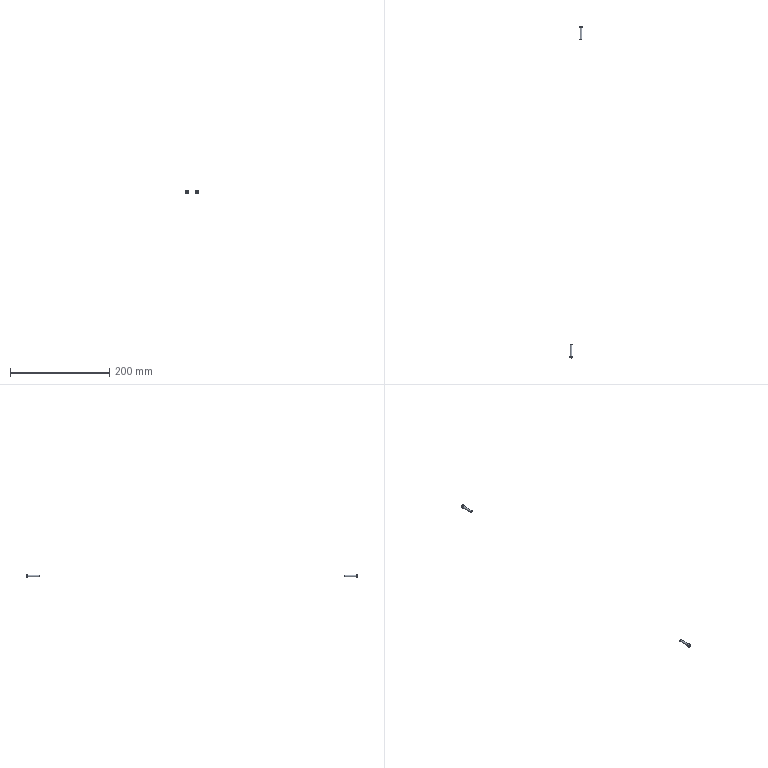Part | STEP file | M4.00-15 | 2 solids | 28 faces | box 27 x 670 x 7 mm | volume 844.151 mm3 | plane 20 | cylinder 4 | cone 4 | commonest cylinder face diameters 4 x2 7 x2